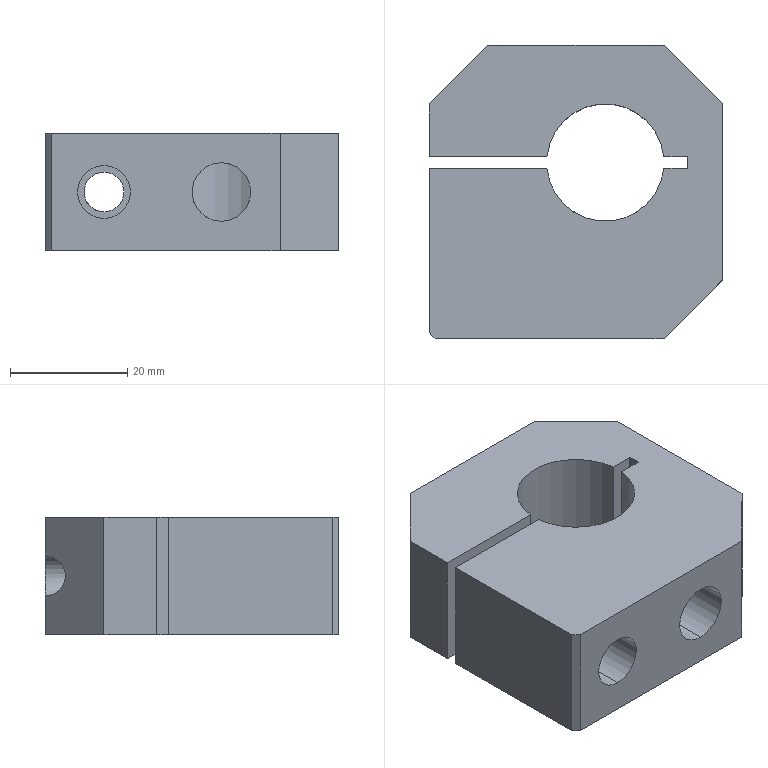Part | SolidWorks | features ICE 3, Chamfer 2, Extrusion 1, HoleWzd 1 | 1 solid | 24 faces | box 50 x 50 x 20 mm | volume 35641 mm3 | plane 16 | cylinder 8 | commonest cylinder face diameters 6.8 x2 9 x2 10 x2 20 x2
STEP:
#1=CARTESIAN_POINT('',(5.,-5.,5.));
#2=VERTEX_POINT('',#1);
#3=CARTESIAN_POINT('',(5.,-5.,15.));
#4=VERTEX_POINT('',#3);
#5=CARTESIAN_POINT('',(5.,-5.,5.));
#6=CARTESIAN_POINT('',(4.664,-5.,5.));
#7=CARTESIAN_POINT('',(4.334,-4.983,5.034));
#8=CARTESIAN_POINT('',(3.686,-4.919,5.164));
#9=CARTESIAN_POINT('',(3.366,-4.87,5.263));
#10=CARTESIAN_POINT('',(2.762,-4.751,5.517));
#11=CARTESIAN_POINT('',(2.477,-4.68,5.671));
#12=CARTESIAN_POINT('',(1.937,-4.524,6.035));
#13=CARTESIAN_POINT('',(1.687,-4.438,6.242));
#14=CARTESIAN_POINT('',(1.234,-4.267,6.695));
#15=CARTESIAN_POINT('',(1.028,-4.179,6.946));
#16=CARTESIAN_POINT('',(0.6671,-4.015,7.484));
#17=CARTESIAN_POINT('',(0.5142,-3.939,7.768));
#18=CARTESIAN_POINT('',(0.3259,-3.841,8.217));
#19=CARTESIAN_POINT('',(0.2701,-3.811,8.371));
#20=CARTESIAN_POINT('',(0.1728,-3.758,8.687));
#21=CARTESIAN_POINT('',(0.1316,-3.735,8.848));
#22=CARTESIAN_POINT('',(0.03353,-3.68,9.334));
#23=CARTESIAN_POINT('',(0.0003238,-3.66,9.662));
#24=CARTESIAN_POINT('',(-0.0001584,-3.66,10.162));
#25=CARTESIAN_POINT('',(0.00812,-3.665,10.33));
#26=CARTESIAN_POINT('',(0.04131,-3.684,10.663));
#27=CARTESIAN_POINT('',(0.06607,-3.698,10.827));
#28=CARTESIAN_POINT('',(0.164,-3.753,11.312));
#29=CARTESIAN_POINT('',(0.2616,-3.807,11.63));
#30=CARTESIAN_POINT('',(0.5153,-3.939,12.235));
#31=CARTESIAN_POINT('',(0.6692,-4.016,12.52));
#32=CARTESIAN_POINT('',(1.03,-4.18,13.057));
#33=CARTESIAN_POINT('',(1.237,-4.268,13.308));
#34=CARTESIAN_POINT('',(1.691,-4.44,13.762));
#35=CARTESIAN_POINT('',(1.939,-4.524,13.967));
#36=CARTESIAN_POINT('',(2.48,-4.681,14.331));
#37=CARTESIAN_POINT('',(2.767,-4.752,14.486));
#38=CARTESIAN_POINT('',(3.217,-4.841,14.674));
#39=CARTESIAN_POINT('',(3.371,-4.868,14.73));
#40=CARTESIAN_POINT('',(3.686,-4.915,14.827));
#41=CARTESIAN_POINT('',(3.848,-4.935,14.868));
#42=CARTESIAN_POINT('',(4.339,-4.984,14.967));
#43=CARTESIAN_POINT('',(4.668,-5.,15.));
#44=CARTESIAN_POINT('',(5.,-5.,15.));
#45=B_SPLINE_CURVE_WITH_KNOTS('',3,(#5,#6,#7,#8,#9,#10,#11,#12,#13,#14,#15,#16,#17,#18,#19,#20,#21,#22,#23,#24,#25,#26,#27,#28,#29,#30,#31,#32,#33,#34,#35,#36,#37,#38,#39,#40,#41,#42,#43,#44),.UNSPECIFIED.,.F.,.F.,(4,2,2,2,2,2,2,2,2,2,2,2,2,2,2,2,2,2,2,4),(0.,0.0009941,0.001988,0.002982,0.003976,0.00497,0.005964,0.006461,0.006958,0.007952,0.008449,0.008947,0.009941,0.01093,0.01193,0.01292,0.01392,0.01441,0.01491,0.0159),.UNSPECIFIED.);
#46=EDGE_CURVE('',#2,#4,#45,.T.);
#47=ORIENTED_EDGE('',*,*,#46,.T.);
#48=CARTESIAN_POINT('',(5.,-25.,15.));
#49=VERTEX_POINT('',#48);
#50=CARTESIAN_POINT('',(5.,1.,15.));
#51=DIRECTION('',(0.,-1.,0.));
#52=VECTOR('',#51,1000.);
#53=LINE('',#50,#52);
#54=EDGE_CURVE('',#4,#49,#53,.T.);
#55=ORIENTED_EDGE('',*,*,#54,.T.);
#56=CARTESIAN_POINT('',(5.,-25.,5.));
#57=VERTEX_POINT('',#56);
#58=CARTESIAN_POINT('',(5.,-25.,10.));
#59=DIRECTION('',(0.,-1.,0.));
#60=DIRECTION('',(0.,0.,-1.));
#61=AXIS2_PLACEMENT_3D('',#58,#59,#60);
#62=CIRCLE('',#61,5.);
#63=EDGE_CURVE('',#49,#57,#62,.T.);
#64=ORIENTED_EDGE('',*,*,#63,.T.);
#65=CARTESIAN_POINT('',(5.,1.,5.));
#66=DIRECTION('',(0.,-1.,0.));
#67=VECTOR('',#66,1000.);
#68=LINE('',#65,#67);
#69=EDGE_CURVE('',#2,#57,#68,.T.);
#70=ORIENTED_EDGE('',*,*,#69,.F.);
#71=EDGE_LOOP('',(#47,#55,#64,#70));
#72=FACE_OUTER_BOUND('',#71,.T.);
#73=CARTESIAN_POINT('',(5.,1.,10.));
#74=DIRECTION('',(0.,-1.,0.));
#75=DIRECTION('',(0.,0.,-1.));
#76=AXIS2_PLACEMENT_3D('',#73,#74,#75);
#77=CYLINDRICAL_SURFACE('',#76,5.);
#78=ADVANCED_FACE('',(#72),#77,.F.);
#79=CARTESIAN_POINT('',(-15.,4.,5.5));
#80=VERTEX_POINT('',#79);
#81=CARTESIAN_POINT('',(-15.,4.,14.5));
#82=VERTEX_POINT('',#81);
#83=CARTESIAN_POINT('',(-15.,4.,10.));
#84=DIRECTION('',(0.,1.,0.));
#85=DIRECTION('',(1.,0.,0.));
#86=AXIS2_PLACEMENT_3D('',#83,#84,#85);
#87=CIRCLE('',#86,4.5);
#88=EDGE_CURVE('',#80,#82,#87,.T.);
#89=ORIENTED_EDGE('',*,*,#88,.T.);
#90=CARTESIAN_POINT('',(-15.,-25.,14.5));
#91=VERTEX_POINT('',#90);
#92=CARTESIAN_POINT('',(-15.,5.,14.5));
#93=DIRECTION('',(0.,-1.,0.));
#94=VECTOR('',#93,1000.);
#95=LINE('',#92,#94);
#96=EDGE_CURVE('',#82,#91,#95,.T.);
#97=ORIENTED_EDGE('',*,*,#96,.T.);
#98=CARTESIAN_POINT('',(-15.,-25.,5.5));
#99=VERTEX_POINT('',#98);
#100=CARTESIAN_POINT('',(-15.,-25.,10.));
#101=DIRECTION('',(0.,-1.,0.));
#102=DIRECTION('',(0.,0.,-1.));
#103=AXIS2_PLACEMENT_3D('',#100,#101,#102);
#104=CIRCLE('',#103,4.5);
#105=EDGE_CURVE('',#91,#99,#104,.T.);
#106=ORIENTED_EDGE('',*,*,#105,.T.);
#107=CARTESIAN_POINT('',(-15.,5.,5.5));
#108=DIRECTION('',(0.,-1.,0.));
#109=VECTOR('',#108,1000.);
#110=LINE('',#107,#109);
#111=EDGE_CURVE('',#80,#99,#110,.T.);
#112=ORIENTED_EDGE('',*,*,#111,.F.);
#113=EDGE_LOOP('',(#89,#97,#106,#112));
#114=FACE_OUTER_BOUND('',#113,.T.);
#115=CARTESIAN_POINT('',(-15.,5.,10.));
#116=DIRECTION('',(0.,-1.,0.));
#117=DIRECTION('',(0.,0.,-1.));
#118=AXIS2_PLACEMENT_3D('',#115,#116,#117);
#119=CYLINDRICAL_SURFACE('',#118,4.5);
#120=ADVANCED_FACE('',(#114),#119,.F.);
#121=CARTESIAN_POINT('',(-15.,6.,13.4));
#122=VERTEX_POINT('',#121);
#123=CARTESIAN_POINT('',(-15.,6.,6.6));
#124=VERTEX_POINT('',#123);
#125=CARTESIAN_POINT('',(-15.,6.,10.));
#126=DIRECTION('',(0.,-1.,0.));
#127=DIRECTION('',(-1.,0.,0.));
#128=AXIS2_PLACEMENT_3D('',#125,#126,#127);
#129=CIRCLE('',#128,3.4);
#130=EDGE_CURVE('',#122,#124,#129,.T.);
#131=ORIENTED_EDGE('',*,*,#130,.T.);
#132=CARTESIAN_POINT('',(-15.,25.,6.6));
#133=VERTEX_POINT('',#132);
#134=CARTESIAN_POINT('',(-15.,25.,6.6));
#135=DIRECTION('',(0.,1.,0.));
#136=VECTOR('',#135,1000.);
#137=LINE('',#134,#136);
#138=EDGE_CURVE('',#124,#133,#137,.T.);
#139=ORIENTED_EDGE('',*,*,#138,.T.);
#140=CARTESIAN_POINT('',(-15.,25.,13.4));
#141=VERTEX_POINT('',#140);
#142=CARTESIAN_POINT('',(-15.,25.,6.6));
#143=CARTESIAN_POINT('',(-21.8,18.2,6.6));
#144=CARTESIAN_POINT('',(-21.8,18.2,13.4));
#145=CARTESIAN_POINT('',(-15.,25.,13.4));
#146=(BOUNDED_CURVE()B_SPLINE_CURVE(3,(#142,#143,#144,#145),.UNSPECIFIED.,.F.,.T.)B_SPLINE_CURVE_WITH_KNOTS((4,4),(1.571,4.712),.UNSPECIFIED.)CURVE()GEOMETRIC_REPRESENTATION_ITEM()RATIONAL_B_SPLINE_CURVE((1.,0.3333,0.3333,1.))REPRESENTATION_ITEM(''));
#147=EDGE_CURVE('',#133,#141,#146,.T.);
#148=ORIENTED_EDGE('',*,*,#147,.T.);
#149=CARTESIAN_POINT('',(-15.,25.,13.4));
#150=DIRECTION('',(0.,1.,0.));
#151=VECTOR('',#150,1000.);
#152=LINE('',#149,#151);
#153=EDGE_CURVE('',#122,#141,#152,.T.);
#154=ORIENTED_EDGE('',*,*,#153,.F.);
#155=EDGE_LOOP('',(#131,#139,#148,#154));
#156=FACE_OUTER_BOUND('',#155,.T.);
#157=CARTESIAN_POINT('',(-15.,25.,10.));
#158=DIRECTION('',(0.,1.,0.));
#159=DIRECTION('',(0.,0.,1.));
#160=AXIS2_PLACEMENT_3D('',#157,#158,#159);
#161=CYLINDRICAL_SURFACE('',#160,3.4);
#162=ADVANCED_FACE('',(#156),#161,.F.);
#163=CARTESIAN_POINT('',(-25.,4.,20.));
#164=VERTEX_POINT('',#163);
#165=CARTESIAN_POINT('',(-25.,-24.,20.));
#166=VERTEX_POINT('',#165);
#167=CARTESIAN_POINT('',(-25.,25.,20.));
#168=DIRECTION('',(0.,-1.,0.));
#169=VECTOR('',#168,1000.);
#170=LINE('',#167,#169);
#171=EDGE_CURVE('',#164,#166,#170,.T.);
#172=ORIENTED_EDGE('',*,*,#171,.F.);
#173=CARTESIAN_POINT('',(-25.,4.,0.));
#174=VERTEX_POINT('',#173);
#175=CARTESIAN_POINT('',(-25.,4.,-7.297));
#176=DIRECTION('',(0.,0.,1.));
#177=VECTOR('',#176,1000.);
#178=LINE('',#175,#177);
#179=EDGE_CURVE('',#174,#164,#178,.T.);
#180=ORIENTED_EDGE('',*,*,#179,.F.);
#181=CARTESIAN_POINT('',(-25.,-24.,0.));
#182=VERTEX_POINT('',#181);
#183=CARTESIAN_POINT('',(-25.,25.,0.));
#184=DIRECTION('',(0.,-1.,0.));
#185=VECTOR('',#184,1000.);
#186=LINE('',#183,#185);
#187=EDGE_CURVE('',#174,#182,#186,.T.);
#188=ORIENTED_EDGE('',*,*,#187,.T.);
#189=CARTESIAN_POINT('',(-25.,-24.,20.));
#190=DIRECTION('',(0.,0.,1.));
#191=VECTOR('',#190,1000.);
#192=LINE('',#189,#191);
#193=EDGE_CURVE('',#182,#166,#192,.T.);
#194=ORIENTED_EDGE('',*,*,#193,.T.);
#195=EDGE_LOOP('',(#172,#180,#188,#194));
#196=FACE_OUTER_BOUND('',#195,.T.);
#197=CARTESIAN_POINT('',(-25.,25.,20.));
#198=DIRECTION('',(1.,0.,0.));
#199=DIRECTION('',(0.,1.,0.));
#200=AXIS2_PLACEMENT_3D('',#197,#198,#199);
#201=PLANE('',#200);
#202=ADVANCED_FACE('',(#196),#201,.F.);
#203=ORIENTED_EDGE('',*,*,#46,.F.);
#204=CARTESIAN_POINT('',(5.,-5.,15.));
#205=CARTESIAN_POINT('',(5.331,-5.,15.));
#206=CARTESIAN_POINT('',(5.669,-4.983,14.966));
#207=CARTESIAN_POINT('',(6.317,-4.918,14.835));
#208=CARTESIAN_POINT('',(6.631,-4.871,14.738));
#209=CARTESIAN_POINT('',(7.24,-4.751,14.482));
#210=CARTESIAN_POINT('',(7.526,-4.68,14.327));
#211=CARTESIAN_POINT('',(8.061,-4.524,13.966));
#212=CARTESIAN_POINT('',(8.314,-4.438,13.758));
#213=CARTESIAN_POINT('',(8.767,-4.266,13.303));
#214=CARTESIAN_POINT('',(8.971,-4.18,13.056));
#215=CARTESIAN_POINT('',(9.331,-4.016,12.52));
#216=CARTESIAN_POINT('',(9.487,-3.938,12.231));
#217=CARTESIAN_POINT('',(9.737,-3.808,11.633));
#218=CARTESIAN_POINT('',(9.834,-3.754,11.321));
#219=CARTESIAN_POINT('',(9.933,-3.699,10.832));
#220=CARTESIAN_POINT('',(9.958,-3.684,10.666));
#221=CARTESIAN_POINT('',(9.991,-3.665,10.336));
#222=CARTESIAN_POINT('',(10.008,-3.656,10.006));
#223=CARTESIAN_POINT('',(9.992,-3.665,9.675));
#224=CARTESIAN_POINT('',(9.959,-3.684,9.343));
#225=CARTESIAN_POINT('',(9.935,-3.698,9.177));
#226=CARTESIAN_POINT('',(9.836,-3.753,8.689));
#227=CARTESIAN_POINT('',(9.74,-3.806,8.375));
#228=CARTESIAN_POINT('',(9.487,-3.938,7.77));
#229=CARTESIAN_POINT('',(9.332,-4.015,7.482));
#230=CARTESIAN_POINT('',(8.973,-4.179,6.947));
#231=CARTESIAN_POINT('',(8.767,-4.267,6.696));
#232=CARTESIAN_POINT('',(8.311,-4.439,6.239));
#233=CARTESIAN_POINT('',(8.064,-4.523,6.035));
#234=CARTESIAN_POINT('',(7.528,-4.679,5.674));
#235=CARTESIAN_POINT('',(7.237,-4.751,5.517));
#236=CARTESIAN_POINT('',(6.635,-4.87,5.264));
#237=CARTESIAN_POINT('',(6.323,-4.918,5.167));
#238=CARTESIAN_POINT('',(5.674,-4.983,5.035));
#239=CARTESIAN_POINT('',(5.336,-5.,5.));
#240=CARTESIAN_POINT('',(5.,-5.,5.));
#241=B_SPLINE_CURVE_WITH_KNOTS('',3,(#204,#205,#206,#207,#208,#209,#210,#211,#212,#213,#214,#215,#216,#217,#218,#219,#220,#221,#222,#223,#224,#225,#226,#227,#228,#229,#230,#231,#232,#233,#234,#235,#236,#237,#238,#239,#240),.UNSPECIFIED.,.F.,.F.,(4,2,2,2,2,2,2,2,2,1,2,2,2,2,2,2,2,2,4),(0.0159,0.0169,0.01789,0.01888,0.01987,0.02087,0.02186,0.02285,0.02335,0.02384,0.02434,0.02484,0.02583,0.02682,0.02781,0.02881,0.0298,0.03079,0.03178),.UNSPECIFIED.);
#242=EDGE_CURVE('',#4,#2,#241,.T.);
#243=ORIENTED_EDGE('',*,*,#242,.F.);
#244=EDGE_LOOP('',(#203,#243));
#245=FACE_BOUND('',#244,.T.);
#246=CARTESIAN_POINT('',(-4.95,4.,20.));
#247=VERTEX_POINT('',#246);
#248=CARTESIAN_POINT('',(-4.95,4.,0.));
#249=VERTEX_POINT('',#248);
#250=CARTESIAN_POINT('',(-4.95,4.,20.));
#251=DIRECTION('',(0.,0.,-1.));
#252=VECTOR('',#251,1000.);
#253=LINE('',#250,#252);
#254=EDGE_CURVE('',#247,#249,#253,.T.);
#255=ORIENTED_EDGE('',*,*,#254,.F.);
#256=CARTESIAN_POINT('',(14.95,4.,20.));
#257=VERTEX_POINT('',#256);
#258=CARTESIAN_POINT('',(5.,5.,20.));
#259=DIRECTION('',(0.,0.,1.));
#260=DIRECTION('',(1.,0.,0.));
#261=AXIS2_PLACEMENT_3D('',#258,#259,#260);
#262=CIRCLE('',#261,10.);
#263=EDGE_CURVE('',#247,#257,#262,.T.);
#264=ORIENTED_EDGE('',*,*,#263,.T.);
#265=CARTESIAN_POINT('',(14.95,4.,0.));
#266=VERTEX_POINT('',#265);
#267=CARTESIAN_POINT('',(14.95,4.,20.));
#268=DIRECTION('',(0.,0.,1.));
#269=VECTOR('',#268,1000.);
#270=LINE('',#267,#269);
#271=EDGE_CURVE('',#266,#257,#270,.T.);
#272=ORIENTED_EDGE('',*,*,#271,.F.);
#273=CARTESIAN_POINT('',(5.,5.,0.));
#274=DIRECTION('',(0.,0.,1.));
#275=DIRECTION('',(1.,0.,0.));
#276=AXIS2_PLACEMENT_3D('',#273,#274,#275);
#277=CIRCLE('',#276,10.);
#278=EDGE_CURVE('',#249,#266,#277,.T.);
#279=ORIENTED_EDGE('',*,*,#278,.F.);
#280=EDGE_LOOP('',(#255,#264,#272,#279));
#281=FACE_OUTER_BOUND('',#280,.T.);
#282=CARTESIAN_POINT('',(5.,5.,20.));
#283=DIRECTION('',(0.,0.,-1.));
#284=DIRECTION('',(-1.,0.,0.));
#285=AXIS2_PLACEMENT_3D('',#282,#283,#284);
#286=CYLINDRICAL_SURFACE('',#285,10.);
#287=ADVANCED_FACE('',(#245,#281),#286,.F.);
#288=ORIENTED_EDGE('',*,*,#138,.F.);
#289=CARTESIAN_POINT('',(-15.,6.,10.));
#290=DIRECTION('',(0.,-1.,0.));
#291=DIRECTION('',(-1.,0.,0.));
#292=AXIS2_PLACEMENT_3D('',#289,#290,#291);
#293=CIRCLE('',#292,3.4);
#294=EDGE_CURVE('',#124,#122,#293,.T.);
#295=ORIENTED_EDGE('',*,*,#294,.T.);
#296=ORIENTED_EDGE('',*,*,#153,.T.);
#297=CARTESIAN_POINT('',(-15.,25.,10.));
#298=DIRECTION('',(0.,1.,0.));
#299=DIRECTION('',(0.,0.,1.));
#300=AXIS2_PLACEMENT_3D('',#297,#298,#299);
#301=CIRCLE('',#300,3.4);
#302=EDGE_CURVE('',#141,#133,#301,.T.);
#303=ORIENTED_EDGE('',*,*,#302,.T.);
#304=EDGE_LOOP('',(#288,#295,#296,#303));
#305=FACE_OUTER_BOUND('',#304,.T.);
#306=CARTESIAN_POINT('',(-15.,25.,10.));
#307=DIRECTION('',(0.,1.,0.));
#308=DIRECTION('',(0.,0.,1.));
#309=AXIS2_PLACEMENT_3D('',#306,#307,#308);
#310=CYLINDRICAL_SURFACE('',#309,3.4);
#311=ADVANCED_FACE('',(#305),#310,.F.);
#312=ORIENTED_EDGE('',*,*,#302,.F.);
#313=CARTESIAN_POINT('',(-15.,25.,20.));
#314=VERTEX_POINT('',#313);
#315=CARTESIAN_POINT('',(-15.,25.,20.));
#316=DIRECTION('',(0.,0.,1.));
#317=VECTOR('',#316,1000.);
#318=LINE('',#315,#317);
#319=EDGE_CURVE('',#141,#314,#318,.T.);
#320=ORIENTED_EDGE('',*,*,#319,.T.);
#321=CARTESIAN_POINT('',(15.,25.,20.));
#322=VERTEX_POINT('',#321);
#323=CARTESIAN_POINT('',(-25.,25.,20.));
#324=DIRECTION('',(-1.,0.,0.));
#325=VECTOR('',#324,1000.);
#326=LINE('',#323,#325);
#327=EDGE_CURVE('',#322,#314,#326,.T.);
#328=ORIENTED_EDGE('',*,*,#327,.F.);
#329=CARTESIAN_POINT('',(15.,25.,0.));
#330=VERTEX_POINT('',#329);
#331=CARTESIAN_POINT('',(15.,25.,20.));
#332=DIRECTION('',(0.,0.,-1.));
#333=VECTOR('',#332,1000.);
#334=LINE('',#331,#333);
#335=EDGE_CURVE('',#322,#330,#334,.T.);
#336=ORIENTED_EDGE('',*,*,#335,.T.);
#337=CARTESIAN_POINT('',(-15.,25.,0.));
#338=VERTEX_POINT('',#337);
#339=CARTESIAN_POINT('',(-25.,25.,0.));
#340=DIRECTION('',(-1.,0.,0.));
#341=VECTOR('',#340,1000.);
#342=LINE('',#339,#341);
#343=EDGE_CURVE('',#330,#338,#342,.T.);
#344=ORIENTED_EDGE('',*,*,#343,.T.);
#345=CARTESIAN_POINT('',(-15.,25.,20.));
#346=DIRECTION('',(0.,0.,1.));
#347=VECTOR('',#346,1000.);
#348=LINE('',#345,#347);
#349=EDGE_CURVE('',#338,#133,#348,.T.);
#350=ORIENTED_EDGE('',*,*,#349,.T.);
#351=EDGE_LOOP('',(#312,#320,#328,#336,#344,#350));
#352=FACE_OUTER_BOUND('',#351,.T.);
#353=CARTESIAN_POINT('',(-25.,25.,20.));
#354=DIRECTION('',(0.,-1.,0.));
#355=DIRECTION('',(0.,0.,-1.));
#356=AXIS2_PLACEMENT_3D('',#353,#354,#355);
#357=PLANE('',#356);
#358=ADVANCED_FACE('',(#352),#357,.F.);
#359=CARTESIAN_POINT('',(0.,4.,20.));
#360=DIRECTION('',(1.,0.,0.));
#361=VECTOR('',#360,1000.);
#362=LINE('',#359,#361);
#363=EDGE_CURVE('',#164,#247,#362,.T.);
#364=ORIENTED_EDGE('',*,*,#363,.F.);
#365=ORIENTED_EDGE('',*,*,#171,.T.);
#366=CARTESIAN_POINT('',(-24.,-25.,20.));
#367=VERTEX_POINT('',#366);
#368=CARTESIAN_POINT('',(-24.5,-24.5,20.));
#369=DIRECTION('',(0.7071,-0.7071,0.));
#370=VECTOR('',#369,1000.);
#371=LINE('',#368,#370);
#372=EDGE_CURVE('',#166,#367,#371,.T.);
#373=ORIENTED_EDGE('',*,*,#372,.T.);
#374=CARTESIAN_POINT('',(15.,-25.,20.));
#375=VERTEX_POINT('',#374);
#376=CARTESIAN_POINT('',(-25.,-25.,20.));
#377=DIRECTION('',(1.,0.,0.));
#378=VECTOR('',#377,1000.);
#379=LINE('',#376,#378);
#380=EDGE_CURVE('',#367,#375,#379,.T.);
#381=ORIENTED_EDGE('',*,*,#380,.T.);
#382=CARTESIAN_POINT('',(25.,-15.,20.));
#383=VERTEX_POINT('',#382);
#384=CARTESIAN_POINT('',(20.,-20.,20.));
#385=DIRECTION('',(0.7071,0.7071,0.));
#386=VECTOR('',#385,1000.);
#387=LINE('',#384,#386);
#388=EDGE_CURVE('',#375,#383,#387,.T.);
#389=ORIENTED_EDGE('',*,*,#388,.T.);
#390=CARTESIAN_POINT('',(25.,15.,20.));
#391=VERTEX_POINT('',#390);
#392=CARTESIAN_POINT('',(25.,25.,20.));
#393=DIRECTION('',(0.,1.,0.));
#394=VECTOR('',#393,1000.);
#395=LINE('',#392,#394);
#396=EDGE_CURVE('',#383,#391,#395,.T.);
#397=ORIENTED_EDGE('',*,*,#396,.T.);
#398=CARTESIAN_POINT('',(20.,20.,20.));
#399=DIRECTION('',(-0.7071,0.7071,0.));
#400=VECTOR('',#399,1000.);
#401=LINE('',#398,#400);
#402=EDGE_CURVE('',#391,#322,#401,.T.);
#403=ORIENTED_EDGE('',*,*,#402,.T.);
#404=ORIENTED_EDGE('',*,*,#327,.T.);
#405=CARTESIAN_POINT('',(-25.,15.,20.));
#406=VERTEX_POINT('',#405);
#407=CARTESIAN_POINT('',(-20.,20.,20.));
#408=DIRECTION('',(-0.7071,-0.7071,0.));
#409=VECTOR('',#408,1000.);
#410=LINE('',#407,#409);
#411=EDGE_CURVE('',#314,#406,#410,.T.);
#412=ORIENTED_EDGE('',*,*,#411,.T.);
#413=CARTESIAN_POINT('',(-25.,6.,20.));
#414=VERTEX_POINT('',#413);
#415=CARTESIAN_POINT('',(-25.,25.,20.));
#416=DIRECTION('',(0.,-1.,0.));
#417=VECTOR('',#416,1000.);
#418=LINE('',#415,#417);
#419=EDGE_CURVE('',#406,#414,#418,.T.);
#420=ORIENTED_EDGE('',*,*,#419,.T.);
#421=CARTESIAN_POINT('',(-4.95,6.,20.));
#422=VERTEX_POINT('',#421);
#423=CARTESIAN_POINT('',(0.,6.,20.));
#424=DIRECTION('',(-1.,0.,0.));
#425=VECTOR('',#424,1000.);
#426=LINE('',#423,#425);
#427=EDGE_CURVE('',#422,#414,#426,.T.);
#428=ORIENTED_EDGE('',*,*,#427,.F.);
#429=CARTESIAN_POINT('',(14.95,6.,20.));
#430=VERTEX_POINT('',#429);
#431=CARTESIAN_POINT('',(5.,5.,20.));
#432=DIRECTION('',(0.,0.,1.));
#433=DIRECTION('',(1.,0.,0.));
#434=AXIS2_PLACEMENT_3D('',#431,#432,#433);
#435=CIRCLE('',#434,10.);
#436=EDGE_CURVE('',#430,#422,#435,.T.);
#437=ORIENTED_EDGE('',*,*,#436,.F.);
#438=CARTESIAN_POINT('',(19.,6.,20.));
#439=VERTEX_POINT('',#438);
#440=CARTESIAN_POINT('',(0.,6.,20.));
#441=DIRECTION('',(-1.,0.,0.));
#442=VECTOR('',#441,1000.);
#443=LINE('',#440,#442);
#444=EDGE_CURVE('',#439,#430,#443,.T.);
#445=ORIENTED_EDGE('',*,*,#444,.F.);
#446=CARTESIAN_POINT('',(19.,4.,20.));
#447=VERTEX_POINT('',#446);
#448=CARTESIAN_POINT('',(19.,0.,20.));
#449=DIRECTION('',(0.,-1.,0.));
#450=VECTOR('',#449,1000.);
#451=LINE('',#448,#450);
#452=EDGE_CURVE('',#439,#447,#451,.T.);
#453=ORIENTED_EDGE('',*,*,#452,.T.);
#454=CARTESIAN_POINT('',(0.,4.,20.));
#455=DIRECTION('',(1.,0.,0.));
#456=VECTOR('',#455,1000.);
#457=LINE('',#454,#456);
#458=EDGE_CURVE('',#257,#447,#457,.T.);
#459=ORIENTED_EDGE('',*,*,#458,.F.);
#460=ORIENTED_EDGE('',*,*,#263,.F.);
#461=EDGE_LOOP('',(#364,#365,#373,#381,#389,#397,#403,#404,#412,#420,#428,#437,#445,#453,#459,#460));
#462=FACE_OUTER_BOUND('',#461,.T.);
#463=CARTESIAN_POINT('',(0.,0.,20.));
#464=DIRECTION('',(0.,0.,1.));
#465=DIRECTION('',(1.,0.,0.));
#466=AXIS2_PLACEMENT_3D('',#463,#464,#465);
#467=PLANE('',#466);
#468=ADVANCED_FACE('',(#462),#467,.T.);
#469=ORIENTED_EDGE('',*,*,#187,.F.);
#470=CARTESIAN_POINT('',(0.,4.,0.));
#471=DIRECTION('',(1.,0.,0.));
#472=VECTOR('',#471,1000.);
#473=LINE('',#470,#472);
#474=EDGE_CURVE('',#174,#249,#473,.T.);
#475=ORIENTED_EDGE('',*,*,#474,.T.);
#476=ORIENTED_EDGE('',*,*,#278,.T.);
#477=CARTESIAN_POINT('',(19.,4.,0.));
#478=VERTEX_POINT('',#477);
#479=CARTESIAN_POINT('',(0.,4.,0.));
#480=DIRECTION('',(1.,0.,0.));
#481=VECTOR('',#480,1000.);
#482=LINE('',#479,#481);
#483=EDGE_CURVE('',#266,#478,#482,.T.);
#484=ORIENTED_EDGE('',*,*,#483,.T.);
#485=CARTESIAN_POINT('',(19.,6.,0.));
#486=VERTEX_POINT('',#485);
#487=CARTESIAN_POINT('',(19.,0.,0.));
#488=DIRECTION('',(0.,-1.,0.));
#489=VECTOR('',#488,1000.);
#490=LINE('',#487,#489);
#491=EDGE_CURVE('',#486,#478,#490,.T.);
#492=ORIENTED_EDGE('',*,*,#491,.F.);
#493=CARTESIAN_POINT('',(14.95,6.,0.));
#494=VERTEX_POINT('',#493);
#495=CARTESIAN_POINT('',(0.,6.,0.));
#496=DIRECTION('',(-1.,0.,0.));
#497=VECTOR('',#496,1000.);
#498=LINE('',#495,#497);
#499=EDGE_CURVE('',#486,#494,#498,.T.);
#500=ORIENTED_EDGE('',*,*,#499,.T.);
#501=CARTESIAN_POINT('',(-4.95,6.,0.));
#502=VERTEX_POINT('',#501);
#503=CARTESIAN_POINT('',(5.,5.,0.));
#504=DIRECTION('',(0.,0.,1.));
#505=DIRECTION('',(1.,0.,0.));
#506=AXIS2_PLACEMENT_3D('',#503,#504,#505);
#507=CIRCLE('',#506,10.);
#508=EDGE_CURVE('',#494,#502,#507,.T.);
#509=ORIENTED_EDGE('',*,*,#508,.T.);
#510=CARTESIAN_POINT('',(-25.,6.,0.));
#511=VERTEX_POINT('',#510);
#512=CARTESIAN_POINT('',(0.,6.,0.));
#513=DIRECTION('',(-1.,0.,0.));
#514=VECTOR('',#513,1000.);
#515=LINE('',#512,#514);
#516=EDGE_CURVE('',#502,#511,#515,.T.);
#517=ORIENTED_EDGE('',*,*,#516,.T.);
#518=CARTESIAN_POINT('',(-25.,15.,0.));
#519=VERTEX_POINT('',#518);
#520=CARTESIAN_POINT('',(-25.,25.,0.));
#521=DIRECTION('',(0.,-1.,0.));
#522=VECTOR('',#521,1000.);
#523=LINE('',#520,#522);
#524=EDGE_CURVE('',#519,#511,#523,.T.);
#525=ORIENTED_EDGE('',*,*,#524,.F.);
#526=CARTESIAN_POINT('',(-25.,15.,0.));
#527=DIRECTION('',(0.7071,0.7071,0.));
#528=VECTOR('',#527,1000.);
#529=LINE('',#526,#528);
#530=EDGE_CURVE('',#519,#338,#529,.T.);
#531=ORIENTED_EDGE('',*,*,#530,.T.);
#532=ORIENTED_EDGE('',*,*,#343,.F.);
#533=CARTESIAN_POINT('',(25.,15.,0.));
#534=VERTEX_POINT('',#533);
#535=CARTESIAN_POINT('',(15.,25.,0.));
#536=DIRECTION('',(0.7071,-0.7071,0.));
#537=VECTOR('',#536,1000.);
#538=LINE('',#535,#537);
#539=EDGE_CURVE('',#330,#534,#538,.T.);
#540=ORIENTED_EDGE('',*,*,#539,.T.);
#541=CARTESIAN_POINT('',(25.,-15.,0.));
#542=VERTEX_POINT('',#541);
#543=CARTESIAN_POINT('',(25.,25.,0.));
#544=DIRECTION('',(0.,1.,0.));
#545=VECTOR('',#544,1000.);
#546=LINE('',#543,#545);
#547=EDGE_CURVE('',#542,#534,#546,.T.);
#548=ORIENTED_EDGE('',*,*,#547,.F.);
#549=CARTESIAN_POINT('',(15.,-25.,0.));
#550=VERTEX_POINT('',#549);
#551=CARTESIAN_POINT('',(25.,-15.,0.));
#552=DIRECTION('',(-0.7071,-0.7071,0.));
#553=VECTOR('',#552,1000.);
#554=LINE('',#551,#553);
#555=EDGE_CURVE('',#542,#550,#554,.T.);
#556=ORIENTED_EDGE('',*,*,#555,.T.);
#557=CARTESIAN_POINT('',(-24.,-25.,0.));
#558=VERTEX_POINT('',#557);
#559=CARTESIAN_POINT('',(-25.,-25.,0.));
#560=DIRECTION('',(1.,0.,0.));
#561=VECTOR('',#560,1000.);
#562=LINE('',#559,#561);
#563=EDGE_CURVE('',#558,#550,#562,.T.);
#564=ORIENTED_EDGE('',*,*,#563,.F.);
#565=CARTESIAN_POINT('',(-24.,-25.,0.));
#566=DIRECTION('',(-0.7071,0.7071,0.));
#567=VECTOR('',#566,1000.);
#568=LINE('',#565,#567);
#569=EDGE_CURVE('',#558,#182,#568,.T.);
#570=ORIENTED_EDGE('',*,*,#569,.T.);
#571=EDGE_LOOP('',(#469,#475,#476,#484,#492,#500,#509,#517,#525,#531,#532,#540,#548,#556,#564,#570));
#572=FACE_OUTER_BOUND('',#571,.T.);
#573=CARTESIAN_POINT('',(0.,0.,0.));
#574=DIRECTION('',(0.,0.,1.));
#575=DIRECTION('',(1.,0.,0.));
#576=AXIS2_PLACEMENT_3D('',#573,#574,#575);
#577=PLANE('',#576);
#578=ADVANCED_FACE('',(#572),#577,.F.);
#579=ORIENTED_EDGE('',*,*,#396,.F.);
#580=CARTESIAN_POINT('',(25.,-15.,20.));
#581=DIRECTION('',(0.,0.,-1.));
#582=VECTOR('',#581,1000.);
#583=LINE('',#580,#582);
#584=EDGE_CURVE('',#383,#542,#583,.T.);
#585=ORIENTED_EDGE('',*,*,#584,.T.);
#586=ORIENTED_EDGE('',*,*,#547,.T.);
#587=CARTESIAN_POINT('',(25.,15.,20.));
#588=DIRECTION('',(0.,0.,1.));
#589=VECTOR('',#588,1000.);
#590=LINE('',#587,#589);
#591=EDGE_CURVE('',#534,#391,#590,.T.);
#592=ORIENTED_EDGE('',*,*,#591,.T.);
#593=EDGE_LOOP('',(#579,#585,#586,#592));
#594=FACE_OUTER_BOUND('',#593,.T.);
#595=CARTESIAN_POINT('',(25.,25.,20.));
#596=DIRECTION('',(-1.,0.,0.));
#597=DIRECTION('',(0.,-1.,0.));
#598=AXIS2_PLACEMENT_3D('',#595,#596,#597);
#599=PLANE('',#598);
#600=ADVANCED_FACE('',(#594),#599,.F.);
#601=ORIENTED_EDGE('',*,*,#524,.T.);
#602=CARTESIAN_POINT('',(-25.,6.,-7.297));
#603=DIRECTION('',(0.,0.,-1.));
#604=VECTOR('',#603,1000.);
#605=LINE('',#602,#604);
#606=EDGE_CURVE('',#414,#511,#605,.T.);
#607=ORIENTED_EDGE('',*,*,#606,.F.);
#608=ORIENTED_EDGE('',*,*,#419,.F.);
#609=CARTESIAN_POINT('',(-25.,15.,20.));
#610=DIRECTION('',(0.,0.,-1.));
#611=VECTOR('',#610,1000.);
#612=LINE('',#609,#611);
#613=EDGE_CURVE('',#406,#519,#612,.T.);
#614=ORIENTED_EDGE('',*,*,#613,.T.);
#615=EDGE_LOOP('',(#601,#607,#608,#614));
#616=FACE_OUTER_BOUND('',#615,.T.);
#617=CARTESIAN_POINT('',(-25.,25.,20.));
#618=DIRECTION('',(1.,0.,0.));
#619=DIRECTION('',(0.,1.,0.));
#620=AXIS2_PLACEMENT_3D('',#617,#618,#619);
#621=PLANE('',#620);
#622=ADVANCED_FACE('',(#616),#621,.F.);
#623=CARTESIAN_POINT('',(5.,-25.,10.));
#624=DIRECTION('',(0.,-1.,0.));
#625=DIRECTION('',(0.,0.,-1.));
#626=AXIS2_PLACEMENT_3D('',#623,#624,#625);
#627=CIRCLE('',#626,5.);
#628=EDGE_CURVE('',#57,#49,#627,.T.);
#629=ORIENTED_EDGE('',*,*,#628,.F.);
#630=ORIENTED_EDGE('',*,*,#63,.F.);
#631=EDGE_LOOP('',(#629,#630));
#632=FACE_BOUND('',#631,.T.);
#633=CARTESIAN_POINT('',(-15.,-25.,10.));
#634=DIRECTION('',(0.,-1.,0.));
#635=DIRECTION('',(0.,0.,-1.));
#636=AXIS2_PLACEMENT_3D('',#633,#634,#635);
#637=CIRCLE('',#636,4.5);
#638=EDGE_CURVE('',#99,#91,#637,.T.);
#639=ORIENTED_EDGE('',*,*,#638,.F.);
#640=ORIENTED_EDGE('',*,*,#105,.F.);
#641=EDGE_LOOP('',(#639,#640));
#642=FACE_BOUND('',#641,.T.);
#643=ORIENTED_EDGE('',*,*,#380,.F.);
#644=CARTESIAN_POINT('',(-24.,-25.,20.));
#645=DIRECTION('',(0.,0.,-1.));
#646=VECTOR('',#645,1000.);
#647=LINE('',#644,#646);
#648=EDGE_CURVE('',#367,#558,#647,.T.);
#649=ORIENTED_EDGE('',*,*,#648,.T.);
#650=ORIENTED_EDGE('',*,*,#563,.T.);
#651=CARTESIAN_POINT('',(15.,-25.,20.));
#652=DIRECTION('',(0.,0.,1.));
#653=VECTOR('',#652,1000.);
#654=LINE('',#651,#653);
#655=EDGE_CURVE('',#550,#375,#654,.T.);
#656=ORIENTED_EDGE('',*,*,#655,.T.);
#657=EDGE_LOOP('',(#643,#649,#650,#656));
#658=FACE_OUTER_BOUND('',#657,.T.);
#659=CARTESIAN_POINT('',(-25.,-25.,20.));
#660=DIRECTION('',(0.,1.,0.));
#661=DIRECTION('',(0.,0.,1.));
#662=AXIS2_PLACEMENT_3D('',#659,#660,#661);
#663=PLANE('',#662);
#664=ADVANCED_FACE('',(#632,#642,#658),#663,.F.);
#665=CARTESIAN_POINT('',(14.95,6.,20.));
#666=DIRECTION('',(0.,0.,-1.));
#667=VECTOR('',#666,1000.);
#668=LINE('',#665,#667);
#669=EDGE_CURVE('',#430,#494,#668,.T.);
#670=ORIENTED_EDGE('',*,*,#669,.F.);
#671=ORIENTED_EDGE('',*,*,#436,.T.);
#672=CARTESIAN_POINT('',(-4.95,6.,20.));
#673=DIRECTION('',(0.,0.,1.));
#674=VECTOR('',#673,1000.);
#675=LINE('',#672,#674);
#676=EDGE_CURVE('',#502,#422,#675,.T.);
#677=ORIENTED_EDGE('',*,*,#676,.F.);
#678=ORIENTED_EDGE('',*,*,#508,.F.);
#679=EDGE_LOOP('',(#670,#671,#677,#678));
#680=FACE_OUTER_BOUND('',#679,.T.);
#681=CARTESIAN_POINT('',(5.,5.,20.));
#682=DIRECTION('',(0.,0.,-1.));
#683=DIRECTION('',(-1.,0.,0.));
#684=AXIS2_PLACEMENT_3D('',#681,#682,#683);
#685=CYLINDRICAL_SURFACE('',#684,10.);
#686=ADVANCED_FACE('',(#680),#685,.F.);
#687=ORIENTED_EDGE('',*,*,#388,.F.);
#688=ORIENTED_EDGE('',*,*,#655,.F.);
#689=ORIENTED_EDGE('',*,*,#555,.F.);
#690=ORIENTED_EDGE('',*,*,#584,.F.);
#691=EDGE_LOOP('',(#687,#688,#689,#690));
#692=FACE_OUTER_BOUND('',#691,.T.);
#693=CARTESIAN_POINT('',(25.,-15.,20.));
#694=DIRECTION('',(-0.7071,0.7071,0.));
#695=DIRECTION('',(0.,0.,-1.));
#696=AXIS2_PLACEMENT_3D('',#693,#694,#695);
#697=PLANE('',#696);
#698=ADVANCED_FACE('',(#692),#697,.F.);
#699=ORIENTED_EDGE('',*,*,#147,.F.);
#700=ORIENTED_EDGE('',*,*,#349,.F.);
#701=ORIENTED_EDGE('',*,*,#530,.F.);
#702=ORIENTED_EDGE('',*,*,#613,.F.);
#703=ORIENTED_EDGE('',*,*,#411,.F.);
#704=ORIENTED_EDGE('',*,*,#319,.F.);
#705=EDGE_LOOP('',(#699,#700,#701,#702,#703,#704));
#706=FACE_OUTER_BOUND('',#705,.T.);
#707=CARTESIAN_POINT('',(-25.,15.,20.));
#708=DIRECTION('',(0.7071,-0.7071,0.));
#709=DIRECTION('',(0.,0.,-1.));
#710=AXIS2_PLACEMENT_3D('',#707,#708,#709);
#711=PLANE('',#710);
#712=ADVANCED_FACE('',(#706),#711,.F.);
#713=ORIENTED_EDGE('',*,*,#402,.F.);
#714=ORIENTED_EDGE('',*,*,#591,.F.);
#715=ORIENTED_EDGE('',*,*,#539,.F.);
#716=ORIENTED_EDGE('',*,*,#335,.F.);
#717=EDGE_LOOP('',(#713,#714,#715,#716));
#718=FACE_OUTER_BOUND('',#717,.T.);
#719=CARTESIAN_POINT('',(15.,25.,20.));
#720=DIRECTION('',(-0.7071,-0.7071,0.));
#721=DIRECTION('',(0.,0.,-1.));
#722=AXIS2_PLACEMENT_3D('',#719,#720,#721);
#723=PLANE('',#722);
#724=ADVANCED_FACE('',(#718),#723,.F.);
#725=ORIENTED_EDGE('',*,*,#372,.F.);
#726=ORIENTED_EDGE('',*,*,#193,.F.);
#727=ORIENTED_EDGE('',*,*,#569,.F.);
#728=ORIENTED_EDGE('',*,*,#648,.F.);
#729=EDGE_LOOP('',(#725,#726,#727,#728));
#730=FACE_OUTER_BOUND('',#729,.T.);
#731=CARTESIAN_POINT('',(-24.,-25.,20.));
#732=DIRECTION('',(0.7071,0.7071,0.));
#733=DIRECTION('',(0.,0.,-1.));
#734=AXIS2_PLACEMENT_3D('',#731,#732,#733);
#735=PLANE('',#734);
#736=ADVANCED_FACE('',(#730),#735,.F.);
#737=ORIENTED_EDGE('',*,*,#96,.F.);
#738=CARTESIAN_POINT('',(-15.,4.,10.));
#739=DIRECTION('',(0.,1.,0.));
#740=DIRECTION('',(1.,0.,0.));
#741=AXIS2_PLACEMENT_3D('',#738,#739,#740);
#742=CIRCLE('',#741,4.5);
#743=EDGE_CURVE('',#82,#80,#742,.T.);
#744=ORIENTED_EDGE('',*,*,#743,.T.);
#745=ORIENTED_EDGE('',*,*,#111,.T.);
#746=ORIENTED_EDGE('',*,*,#638,.T.);
#747=EDGE_LOOP('',(#737,#744,#745,#746));
#748=FACE_OUTER_BOUND('',#747,.T.);
#749=CARTESIAN_POINT('',(-15.,5.,10.));
#750=DIRECTION('',(0.,-1.,0.));
#751=DIRECTION('',(0.,0.,-1.));
#752=AXIS2_PLACEMENT_3D('',#749,#750,#751);
#753=CYLINDRICAL_SURFACE('',#752,4.5);
#754=ADVANCED_FACE('',(#748),#753,.F.);
#755=ORIENTED_EDGE('',*,*,#363,.T.);
#756=ORIENTED_EDGE('',*,*,#254,.T.);
#757=ORIENTED_EDGE('',*,*,#474,.F.);
#758=ORIENTED_EDGE('',*,*,#179,.T.);
#759=EDGE_LOOP('',(#755,#756,#757,#758));
#760=FACE_OUTER_BOUND('',#759,.T.);
#761=ORIENTED_EDGE('',*,*,#88,.F.);
#762=ORIENTED_EDGE('',*,*,#743,.F.);
#763=EDGE_LOOP('',(#761,#762));
#764=FACE_BOUND('',#763,.T.);
#765=CARTESIAN_POINT('',(19.,4.,-7.297));
#766=DIRECTION('',(0.,-1.,0.));
#767=DIRECTION('',(1.,0.,0.));
#768=AXIS2_PLACEMENT_3D('',#765,#766,#767);
#769=PLANE('',#768);
#770=ADVANCED_FACE('',(#760,#764),#769,.F.);
#771=ORIENTED_EDGE('',*,*,#427,.T.);
#772=ORIENTED_EDGE('',*,*,#606,.T.);
#773=ORIENTED_EDGE('',*,*,#516,.F.);
#774=ORIENTED_EDGE('',*,*,#676,.T.);
#775=EDGE_LOOP('',(#771,#772,#773,#774));
#776=FACE_OUTER_BOUND('',#775,.T.);
#777=ORIENTED_EDGE('',*,*,#130,.F.);
#778=ORIENTED_EDGE('',*,*,#294,.F.);
#779=EDGE_LOOP('',(#777,#778));
#780=FACE_BOUND('',#779,.T.);
#781=CARTESIAN_POINT('',(19.,6.,-7.297));
#782=DIRECTION('',(0.,1.,0.));
#783=DIRECTION('',(-1.,0.,0.));
#784=AXIS2_PLACEMENT_3D('',#781,#782,#783);
#785=PLANE('',#784);
#786=ADVANCED_FACE('',(#776,#780),#785,.F.);
#787=CARTESIAN_POINT('',(19.,6.,-7.297));
#788=DIRECTION('',(0.,0.,-1.));
#789=VECTOR('',#788,1000.);
#790=LINE('',#787,#789);
#791=EDGE_CURVE('',#439,#486,#790,.T.);
#792=ORIENTED_EDGE('',*,*,#791,.T.);
#793=ORIENTED_EDGE('',*,*,#491,.T.);
#794=CARTESIAN_POINT('',(19.,4.,-7.297));
#795=DIRECTION('',(0.,0.,1.));
#796=VECTOR('',#795,1000.);
#797=LINE('',#794,#796);
#798=EDGE_CURVE('',#478,#447,#797,.T.);
#799=ORIENTED_EDGE('',*,*,#798,.T.);
#800=ORIENTED_EDGE('',*,*,#452,.F.);
#801=EDGE_LOOP('',(#792,#793,#799,#800));
#802=FACE_OUTER_BOUND('',#801,.T.);
#803=CARTESIAN_POINT('',(19.,0.,0.));
#804=DIRECTION('',(-1.,0.,0.));
#805=DIRECTION('',(0.,0.,1.));
#806=AXIS2_PLACEMENT_3D('',#803,#804,#805);
#807=PLANE('',#806);
#808=ADVANCED_FACE('',(#802),#807,.T.);
#809=ORIENTED_EDGE('',*,*,#444,.T.);
#810=ORIENTED_EDGE('',*,*,#669,.T.);
#811=ORIENTED_EDGE('',*,*,#499,.F.);
#812=ORIENTED_EDGE('',*,*,#791,.F.);
#813=EDGE_LOOP('',(#809,#810,#811,#812));
#814=FACE_OUTER_BOUND('',#813,.T.);
#815=CARTESIAN_POINT('',(19.,6.,-7.297));
#816=DIRECTION('',(0.,1.,0.));
#817=DIRECTION('',(-1.,0.,0.));
#818=AXIS2_PLACEMENT_3D('',#815,#816,#817);
#819=PLANE('',#818);
#820=ADVANCED_FACE('',(#814),#819,.F.);
#821=ORIENTED_EDGE('',*,*,#458,.T.);
#822=ORIENTED_EDGE('',*,*,#798,.F.);
#823=ORIENTED_EDGE('',*,*,#483,.F.);
#824=ORIENTED_EDGE('',*,*,#271,.T.);
#825=EDGE_LOOP('',(#821,#822,#823,#824));
#826=FACE_OUTER_BOUND('',#825,.T.);
#827=CARTESIAN_POINT('',(19.,4.,-7.297));
#828=DIRECTION('',(0.,-1.,0.));
#829=DIRECTION('',(1.,0.,0.));
#830=AXIS2_PLACEMENT_3D('',#827,#828,#829);
#831=PLANE('',#830);
#832=ADVANCED_FACE('',(#826),#831,.F.);
#833=ORIENTED_EDGE('',*,*,#54,.F.);
#834=ORIENTED_EDGE('',*,*,#242,.T.);
#835=ORIENTED_EDGE('',*,*,#69,.T.);
#836=ORIENTED_EDGE('',*,*,#628,.T.);
#837=EDGE_LOOP('',(#833,#834,#835,#836));
#838=FACE_OUTER_BOUND('',#837,.T.);
#839=CARTESIAN_POINT('',(5.,1.,10.));
#840=DIRECTION('',(0.,-1.,0.));
#841=DIRECTION('',(0.,0.,-1.));
#842=AXIS2_PLACEMENT_3D('',#839,#840,#841);
#843=CYLINDRICAL_SURFACE('',#842,5.);
#844=ADVANCED_FACE('',(#838),#843,.F.);
#845=CLOSED_SHELL('',(#78,#120,#162,#202,#287,#311,#358,#468,#578,#600,#622,#664,#686,#698,#712,#724,#736,#754,#770,#786,#808,#820,#832,#844));
#846=MANIFOLD_SOLID_BREP('',#845);
#847=CARTESIAN_POINT('',(0.,0.,0.));
#848=DIRECTION('',(0.,0.,1.));
#849=DIRECTION('',(1.,0.,0.));
#850=AXIS2_PLACEMENT_3D('',#847,#848,#849);
#851=(LENGTH_UNIT()NAMED_UNIT(*)SI_UNIT(.MILLI.,.METRE.));
#852=UNCERTAINTY_MEASURE_WITH_UNIT(LENGTH_MEASURE(0.00001),#851,'','');
#853=(NAMED_UNIT(*)PLANE_ANGLE_UNIT()SI_UNIT($,.RADIAN.));
#854=(NAMED_UNIT(*)SI_UNIT($,.STERADIAN.)SOLID_ANGLE_UNIT());
#855=(GEOMETRIC_REPRESENTATION_CONTEXT(3)GLOBAL_UNCERTAINTY_ASSIGNED_CONTEXT((#852))GLOBAL_UNIT_ASSIGNED_CONTEXT((#851,#853,#854))REPRESENTATION_CONTEXT('',''));
#856=ADVANCED_BREP_SHAPE_REPRESENTATION('',(#846,#850),#855);